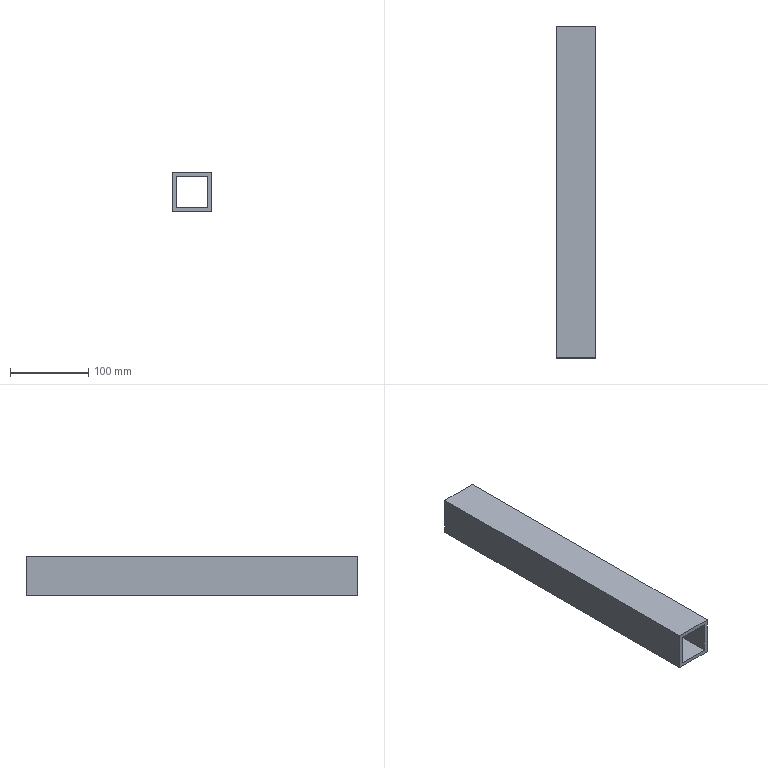Part | NX | features solid 2 | 1 solid | 10 faces | box 50 x 425 x 50 mm | volume 382500 mm3 | plane 10
STEP:
#1=CARTESIAN_POINT('',(585.,50.,1250.));
#2=VERTEX_POINT('',#1);
#3=CARTESIAN_POINT('',(625.,50.,1250.));
#4=VERTEX_POINT('',#3);
#5=CARTESIAN_POINT('',(630.,50.,1250.));
#6=DIRECTION('',(1.,0.,0.));
#7=VECTOR('',#6,1000.);
#8=LINE('',#5,#7);
#9=EDGE_CURVE('',#2,#4,#8,.T.);
#10=ORIENTED_EDGE('',*,*,#9,.F.);
#11=CARTESIAN_POINT('',(585.,50.,1290.));
#12=VERTEX_POINT('',#11);
#13=CARTESIAN_POINT('',(585.,50.,1245.));
#14=DIRECTION('',(0.,0.,-1.));
#15=VECTOR('',#14,1000.);
#16=LINE('',#13,#15);
#17=EDGE_CURVE('',#12,#2,#16,.T.);
#18=ORIENTED_EDGE('',*,*,#17,.F.);
#19=CARTESIAN_POINT('',(625.,50.,1290.));
#20=VERTEX_POINT('',#19);
#21=CARTESIAN_POINT('',(630.,50.,1290.));
#22=DIRECTION('',(-1.,0.,0.));
#23=VECTOR('',#22,1000.);
#24=LINE('',#21,#23);
#25=EDGE_CURVE('',#20,#12,#24,.T.);
#26=ORIENTED_EDGE('',*,*,#25,.F.);
#27=CARTESIAN_POINT('',(625.,50.,1245.));
#28=DIRECTION('',(0.,0.,1.));
#29=VECTOR('',#28,1000.);
#30=LINE('',#27,#29);
#31=EDGE_CURVE('',#4,#20,#30,.T.);
#32=ORIENTED_EDGE('',*,*,#31,.F.);
#33=EDGE_LOOP('',(#10,#18,#26,#32));
#34=FACE_BOUND('',#33,.T.);
#35=CARTESIAN_POINT('',(630.,50.,1295.));
#36=VERTEX_POINT('',#35);
#37=CARTESIAN_POINT('',(580.,50.,1295.));
#38=VERTEX_POINT('',#37);
#39=CARTESIAN_POINT('',(630.,50.,1295.));
#40=DIRECTION('',(-1.,0.,0.));
#41=VECTOR('',#40,1000.);
#42=LINE('',#39,#41);
#43=EDGE_CURVE('',#36,#38,#42,.T.);
#44=ORIENTED_EDGE('',*,*,#43,.T.);
#45=CARTESIAN_POINT('',(580.,50.,1245.));
#46=VERTEX_POINT('',#45);
#47=CARTESIAN_POINT('',(580.,50.,1245.));
#48=DIRECTION('',(0.,0.,-1.));
#49=VECTOR('',#48,1000.);
#50=LINE('',#47,#49);
#51=EDGE_CURVE('',#38,#46,#50,.T.);
#52=ORIENTED_EDGE('',*,*,#51,.T.);
#53=CARTESIAN_POINT('',(630.,50.,1245.));
#54=VERTEX_POINT('',#53);
#55=CARTESIAN_POINT('',(630.,50.,1245.));
#56=DIRECTION('',(1.,0.,0.));
#57=VECTOR('',#56,1000.);
#58=LINE('',#55,#57);
#59=EDGE_CURVE('',#46,#54,#58,.T.);
#60=ORIENTED_EDGE('',*,*,#59,.T.);
#61=CARTESIAN_POINT('',(630.,50.,1245.));
#62=DIRECTION('',(0.,0.,1.));
#63=VECTOR('',#62,1000.);
#64=LINE('',#61,#63);
#65=EDGE_CURVE('',#54,#36,#64,.T.);
#66=ORIENTED_EDGE('',*,*,#65,.T.);
#67=EDGE_LOOP('',(#44,#52,#60,#66));
#68=FACE_BOUND('',#67,.T.);
#69=CARTESIAN_POINT('',(630.,50.,1245.));
#70=DIRECTION('',(0.,1.,0.));
#71=DIRECTION('',(1.,0.,0.));
#72=AXIS2_PLACEMENT_3D('',#69,#70,#71);
#73=PLANE('',#72);
#74=ADVANCED_FACE('',(#34,#68),#73,.F.);
#75=CARTESIAN_POINT('',(630.,475.,1245.));
#76=VERTEX_POINT('',#75);
#77=CARTESIAN_POINT('',(630.,50.,1245.));
#78=DIRECTION('',(0.,1.,0.));
#79=VECTOR('',#78,1000.);
#80=LINE('',#77,#79);
#81=EDGE_CURVE('',#54,#76,#80,.T.);
#82=ORIENTED_EDGE('',*,*,#81,.T.);
#83=CARTESIAN_POINT('',(630.,475.,1295.));
#84=VERTEX_POINT('',#83);
#85=CARTESIAN_POINT('',(630.,475.,1245.));
#86=DIRECTION('',(0.,0.,-1.));
#87=VECTOR('',#86,1000.);
#88=LINE('',#85,#87);
#89=EDGE_CURVE('',#84,#76,#88,.T.);
#90=ORIENTED_EDGE('',*,*,#89,.F.);
#91=CARTESIAN_POINT('',(630.,50.,1295.));
#92=DIRECTION('',(0.,-1.,0.));
#93=VECTOR('',#92,1000.);
#94=LINE('',#91,#93);
#95=EDGE_CURVE('',#84,#36,#94,.T.);
#96=ORIENTED_EDGE('',*,*,#95,.T.);
#97=ORIENTED_EDGE('',*,*,#65,.F.);
#98=EDGE_LOOP('',(#82,#90,#96,#97));
#99=FACE_BOUND('',#98,.T.);
#100=CARTESIAN_POINT('',(630.,50.,1245.));
#101=DIRECTION('',(-1.,0.,0.));
#102=DIRECTION('',(0.,0.,1.));
#103=AXIS2_PLACEMENT_3D('',#100,#101,#102);
#104=PLANE('',#103);
#105=ADVANCED_FACE('',(#99),#104,.F.);
#106=CARTESIAN_POINT('',(580.,475.,1245.));
#107=VERTEX_POINT('',#106);
#108=CARTESIAN_POINT('',(580.,50.,1245.));
#109=DIRECTION('',(0.,1.,0.));
#110=VECTOR('',#109,1000.);
#111=LINE('',#108,#110);
#112=EDGE_CURVE('',#46,#107,#111,.T.);
#113=ORIENTED_EDGE('',*,*,#112,.T.);
#114=CARTESIAN_POINT('',(630.,475.,1245.));
#115=DIRECTION('',(-1.,0.,0.));
#116=VECTOR('',#115,1000.);
#117=LINE('',#114,#116);
#118=EDGE_CURVE('',#76,#107,#117,.T.);
#119=ORIENTED_EDGE('',*,*,#118,.F.);
#120=ORIENTED_EDGE('',*,*,#81,.F.);
#121=ORIENTED_EDGE('',*,*,#59,.F.);
#122=EDGE_LOOP('',(#113,#119,#120,#121));
#123=FACE_BOUND('',#122,.T.);
#124=CARTESIAN_POINT('',(630.,50.,1245.));
#125=DIRECTION('',(0.,0.,1.));
#126=DIRECTION('',(0.,-1.,0.));
#127=AXIS2_PLACEMENT_3D('',#124,#125,#126);
#128=PLANE('',#127);
#129=ADVANCED_FACE('',(#123),#128,.F.);
#130=CARTESIAN_POINT('',(580.,475.,1295.));
#131=VERTEX_POINT('',#130);
#132=CARTESIAN_POINT('',(580.,50.,1295.));
#133=DIRECTION('',(0.,1.,0.));
#134=VECTOR('',#133,1000.);
#135=LINE('',#132,#134);
#136=EDGE_CURVE('',#38,#131,#135,.T.);
#137=ORIENTED_EDGE('',*,*,#136,.T.);
#138=CARTESIAN_POINT('',(580.,475.,1295.));
#139=DIRECTION('',(0.,0.,1.));
#140=VECTOR('',#139,1000.);
#141=LINE('',#138,#140);
#142=EDGE_CURVE('',#107,#131,#141,.T.);
#143=ORIENTED_EDGE('',*,*,#142,.F.);
#144=ORIENTED_EDGE('',*,*,#112,.F.);
#145=ORIENTED_EDGE('',*,*,#51,.F.);
#146=EDGE_LOOP('',(#137,#143,#144,#145));
#147=FACE_BOUND('',#146,.T.);
#148=CARTESIAN_POINT('',(580.,50.,1295.));
#149=DIRECTION('',(1.,0.,0.));
#150=DIRECTION('',(0.,-1.,0.));
#151=AXIS2_PLACEMENT_3D('',#148,#149,#150);
#152=PLANE('',#151);
#153=ADVANCED_FACE('',(#147),#152,.F.);
#154=ORIENTED_EDGE('',*,*,#95,.F.);
#155=CARTESIAN_POINT('',(630.,475.,1295.));
#156=DIRECTION('',(1.,0.,0.));
#157=VECTOR('',#156,1000.);
#158=LINE('',#155,#157);
#159=EDGE_CURVE('',#131,#84,#158,.T.);
#160=ORIENTED_EDGE('',*,*,#159,.F.);
#161=ORIENTED_EDGE('',*,*,#136,.F.);
#162=ORIENTED_EDGE('',*,*,#43,.F.);
#163=EDGE_LOOP('',(#154,#160,#161,#162));
#164=FACE_BOUND('',#163,.T.);
#165=CARTESIAN_POINT('',(630.,480.,1295.));
#166=DIRECTION('',(0.,0.,-1.));
#167=DIRECTION('',(-1.,0.,0.));
#168=AXIS2_PLACEMENT_3D('',#165,#166,#167);
#169=PLANE('',#168);
#170=ADVANCED_FACE('',(#164),#169,.F.);
#171=CARTESIAN_POINT('',(585.,475.,1250.));
#172=VERTEX_POINT('',#171);
#173=CARTESIAN_POINT('',(625.,475.,1250.));
#174=VERTEX_POINT('',#173);
#175=CARTESIAN_POINT('',(630.,475.,1250.));
#176=DIRECTION('',(1.,0.,0.));
#177=VECTOR('',#176,1000.);
#178=LINE('',#175,#177);
#179=EDGE_CURVE('',#172,#174,#178,.T.);
#180=ORIENTED_EDGE('',*,*,#179,.F.);
#181=CARTESIAN_POINT('',(585.,50.,1250.));
#182=DIRECTION('',(0.,1.,0.));
#183=VECTOR('',#182,1000.);
#184=LINE('',#181,#183);
#185=EDGE_CURVE('',#2,#172,#184,.T.);
#186=ORIENTED_EDGE('',*,*,#185,.F.);
#187=ORIENTED_EDGE('',*,*,#9,.T.);
#188=CARTESIAN_POINT('',(625.,50.,1250.));
#189=DIRECTION('',(0.,-1.,0.));
#190=VECTOR('',#189,1000.);
#191=LINE('',#188,#190);
#192=EDGE_CURVE('',#174,#4,#191,.T.);
#193=ORIENTED_EDGE('',*,*,#192,.F.);
#194=EDGE_LOOP('',(#180,#186,#187,#193));
#195=FACE_BOUND('',#194,.T.);
#196=CARTESIAN_POINT('',(585.,50.,1250.));
#197=DIRECTION('',(0.,0.,1.));
#198=DIRECTION('',(0.,-1.,0.));
#199=AXIS2_PLACEMENT_3D('',#196,#197,#198);
#200=PLANE('',#199);
#201=ADVANCED_FACE('',(#195),#200,.T.);
#202=CARTESIAN_POINT('',(625.,475.,1290.));
#203=VERTEX_POINT('',#202);
#204=CARTESIAN_POINT('',(625.,475.,1245.));
#205=DIRECTION('',(0.,0.,1.));
#206=VECTOR('',#205,1000.);
#207=LINE('',#204,#206);
#208=EDGE_CURVE('',#174,#203,#207,.T.);
#209=ORIENTED_EDGE('',*,*,#208,.F.);
#210=ORIENTED_EDGE('',*,*,#192,.T.);
#211=ORIENTED_EDGE('',*,*,#31,.T.);
#212=CARTESIAN_POINT('',(625.,480.,1290.));
#213=DIRECTION('',(0.,-1.,0.));
#214=VECTOR('',#213,1000.);
#215=LINE('',#212,#214);
#216=EDGE_CURVE('',#203,#20,#215,.T.);
#217=ORIENTED_EDGE('',*,*,#216,.F.);
#218=EDGE_LOOP('',(#209,#210,#211,#217));
#219=FACE_BOUND('',#218,.T.);
#220=CARTESIAN_POINT('',(625.,480.,1250.));
#221=DIRECTION('',(-1.,0.,0.));
#222=DIRECTION('',(0.,0.,1.));
#223=AXIS2_PLACEMENT_3D('',#220,#221,#222);
#224=PLANE('',#223);
#225=ADVANCED_FACE('',(#219),#224,.T.);
#226=CARTESIAN_POINT('',(585.,475.,1290.));
#227=VERTEX_POINT('',#226);
#228=CARTESIAN_POINT('',(630.,475.,1290.));
#229=DIRECTION('',(-1.,0.,0.));
#230=VECTOR('',#229,1000.);
#231=LINE('',#228,#230);
#232=EDGE_CURVE('',#203,#227,#231,.T.);
#233=ORIENTED_EDGE('',*,*,#232,.F.);
#234=ORIENTED_EDGE('',*,*,#216,.T.);
#235=ORIENTED_EDGE('',*,*,#25,.T.);
#236=CARTESIAN_POINT('',(585.,480.,1290.));
#237=DIRECTION('',(0.,-1.,0.));
#238=VECTOR('',#237,1000.);
#239=LINE('',#236,#238);
#240=EDGE_CURVE('',#227,#12,#239,.T.);
#241=ORIENTED_EDGE('',*,*,#240,.F.);
#242=EDGE_LOOP('',(#233,#234,#235,#241));
#243=FACE_BOUND('',#242,.T.);
#244=CARTESIAN_POINT('',(625.,480.,1290.));
#245=DIRECTION('',(0.,0.,-1.));
#246=DIRECTION('',(-1.,0.,0.));
#247=AXIS2_PLACEMENT_3D('',#244,#245,#246);
#248=PLANE('',#247);
#249=ADVANCED_FACE('',(#243),#248,.T.);
#250=CARTESIAN_POINT('',(585.,475.,1245.));
#251=DIRECTION('',(0.,0.,-1.));
#252=VECTOR('',#251,1000.);
#253=LINE('',#250,#252);
#254=EDGE_CURVE('',#227,#172,#253,.T.);
#255=ORIENTED_EDGE('',*,*,#254,.F.);
#256=ORIENTED_EDGE('',*,*,#240,.T.);
#257=ORIENTED_EDGE('',*,*,#17,.T.);
#258=ORIENTED_EDGE('',*,*,#185,.T.);
#259=EDGE_LOOP('',(#255,#256,#257,#258));
#260=FACE_BOUND('',#259,.T.);
#261=CARTESIAN_POINT('',(585.,50.,1290.));
#262=DIRECTION('',(1.,0.,0.));
#263=DIRECTION('',(0.,-1.,0.));
#264=AXIS2_PLACEMENT_3D('',#261,#262,#263);
#265=PLANE('',#264);
#266=ADVANCED_FACE('',(#260),#265,.T.);
#267=ORIENTED_EDGE('',*,*,#232,.T.);
#268=ORIENTED_EDGE('',*,*,#254,.T.);
#269=ORIENTED_EDGE('',*,*,#179,.T.);
#270=ORIENTED_EDGE('',*,*,#208,.T.);
#271=EDGE_LOOP('',(#267,#268,#269,#270));
#272=FACE_BOUND('',#271,.T.);
#273=ORIENTED_EDGE('',*,*,#142,.T.);
#274=ORIENTED_EDGE('',*,*,#159,.T.);
#275=ORIENTED_EDGE('',*,*,#89,.T.);
#276=ORIENTED_EDGE('',*,*,#118,.T.);
#277=EDGE_LOOP('',(#273,#274,#275,#276));
#278=FACE_BOUND('',#277,.T.);
#279=CARTESIAN_POINT('',(630.,475.,1245.));
#280=DIRECTION('',(0.,1.,0.));
#281=DIRECTION('',(1.,0.,0.));
#282=AXIS2_PLACEMENT_3D('',#279,#280,#281);
#283=PLANE('',#282);
#284=ADVANCED_FACE('',(#272,#278),#283,.T.);
#285=CLOSED_SHELL('',(#74,#105,#129,#153,#170,#201,#225,#249,#266,#284));
#286=MANIFOLD_SOLID_BREP('',#285);
#287=(LENGTH_UNIT()NAMED_UNIT(*)SI_UNIT(.MILLI.,.METRE.));
#288=UNCERTAINTY_MEASURE_WITH_UNIT(LENGTH_MEASURE(0.00001),#287,'','');
#289=(NAMED_UNIT(*)PLANE_ANGLE_UNIT()SI_UNIT($,.RADIAN.));
#290=(NAMED_UNIT(*)SI_UNIT($,.STERADIAN.)SOLID_ANGLE_UNIT());
#291=(GEOMETRIC_REPRESENTATION_CONTEXT(3)GLOBAL_UNCERTAINTY_ASSIGNED_CONTEXT((#288))GLOBAL_UNIT_ASSIGNED_CONTEXT((#287,#289,#290))REPRESENTATION_CONTEXT('',''));
#292=ADVANCED_BREP_SHAPE_REPRESENTATION('',(#286),#291);